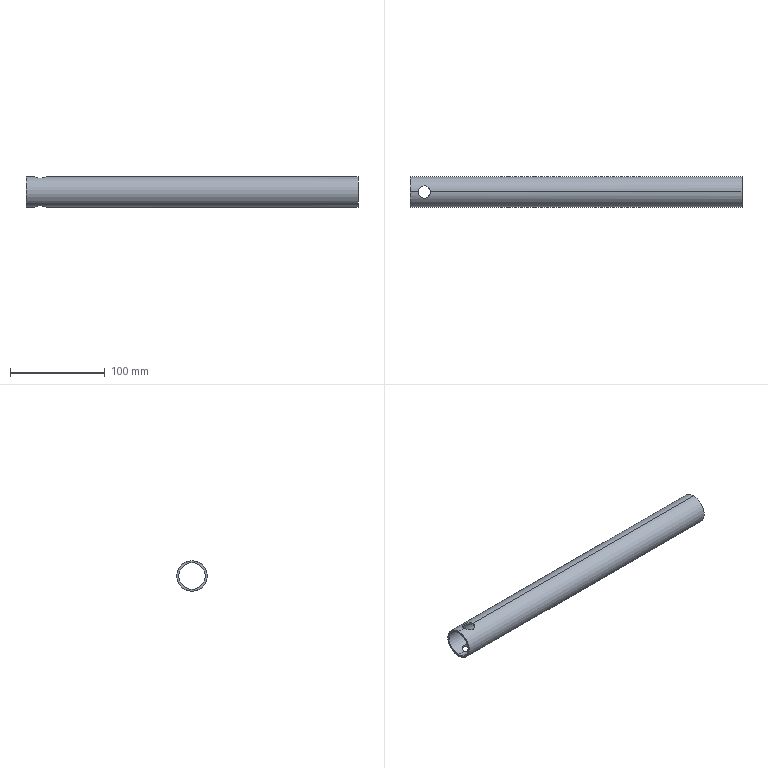Part | SolidWorks | features ICE 1, Sweep 1 | 1 solid | 10 faces | box 350 x 32 x 32 mm | volume 65429 mm3 | cylinder 8 | plane 2 | commonest cylinder face diameters 13 x4 28 x2 32 x2
STEP:
#1=CARTESIAN_POINT('',(-153.5,0.,-16.));
#2=VERTEX_POINT('',#1);
#3=CARTESIAN_POINT('',(-166.5,0.,-16.));
#4=VERTEX_POINT('',#3);
#5=CARTESIAN_POINT('',(-153.5,0.,-16.));
#6=CARTESIAN_POINT('',(-153.5,-0.4345,-16.));
#7=CARTESIAN_POINT('',(-153.543,-0.8609,-15.982));
#8=CARTESIAN_POINT('',(-153.669,-1.489,-15.932));
#9=CARTESIAN_POINT('',(-153.722,-1.696,-15.911));
#10=CARTESIAN_POINT('',(-153.847,-2.107,-15.862));
#11=CARTESIAN_POINT('',(-153.921,-2.31,-15.834));
#12=CARTESIAN_POINT('',(-154.167,-2.899,-15.74));
#13=CARTESIAN_POINT('',(-154.367,-3.271,-15.666));
#14=CARTESIAN_POINT('',(-154.721,-3.798,-15.544));
#15=CARTESIAN_POINT('',(-154.849,-3.97,-15.501));
#16=CARTESIAN_POINT('',(-155.117,-4.296,-15.413));
#17=CARTESIAN_POINT('',(-155.259,-4.451,-15.369));
#18=CARTESIAN_POINT('',(-155.703,-4.895,-15.236));
#19=CARTESIAN_POINT('',(-156.029,-5.164,-15.146));
#20=CARTESIAN_POINT('',(-156.735,-5.637,-14.976));
#21=CARTESIAN_POINT('',(-157.106,-5.836,-14.899));
#22=CARTESIAN_POINT('',(-157.691,-6.08,-14.8));
#23=CARTESIAN_POINT('',(-157.891,-6.152,-14.77));
#24=CARTESIAN_POINT('',(-158.3,-6.278,-14.717));
#25=CARTESIAN_POINT('',(-158.511,-6.331,-14.694));
#26=CARTESIAN_POINT('',(-159.142,-6.457,-14.639));
#27=CARTESIAN_POINT('',(-159.567,-6.5,-14.62));
#28=CARTESIAN_POINT('',(-160.425,-6.5,-14.62));
#29=CARTESIAN_POINT('',(-160.861,-6.457,-14.64));
#30=CARTESIAN_POINT('',(-161.699,-6.289,-14.713));
#31=CARTESIAN_POINT('',(-162.108,-6.164,-14.766));
#32=CARTESIAN_POINT('',(-162.899,-5.833,-14.9));
#33=CARTESIAN_POINT('',(-163.271,-5.633,-14.978));
#34=CARTESIAN_POINT('',(-163.97,-5.164,-15.146));
#35=CARTESIAN_POINT('',(-164.301,-4.892,-15.237));
#36=CARTESIAN_POINT('',(-164.895,-4.297,-15.415));
#37=CARTESIAN_POINT('',(-165.161,-3.973,-15.503));
#38=CARTESIAN_POINT('',(-165.515,-3.447,-15.625));
#39=CARTESIAN_POINT('',(-165.626,-3.263,-15.665));
#40=CARTESIAN_POINT('',(-165.827,-2.888,-15.738));
#41=CARTESIAN_POINT('',(-165.918,-2.697,-15.772));
#42=CARTESIAN_POINT('',(-166.162,-2.111,-15.865));
#43=CARTESIAN_POINT('',(-166.287,-1.704,-15.915));
#44=CARTESIAN_POINT('',(-166.458,-0.8569,-15.983));
#45=CARTESIAN_POINT('',(-166.5,-0.428,-16.));
#46=CARTESIAN_POINT('',(-166.5,0.,-16.));
#47=B_SPLINE_CURVE_WITH_KNOTS('',3,(#5,#6,#7,#8,#9,#10,#11,#12,#13,#14,#15,#16,#17,#18,#19,#20,#21,#22,#23,#24,#25,#26,#27,#28,#29,#30,#31,#32,#33,#34,#35,#36,#37,#38,#39,#40,#41,#42,#43,#44,#45,#46),.UNSPECIFIED.,.F.,.F.,(4,2,2,2,2,2,2,2,2,2,2,2,2,2,2,2,2,2,2,2,4),(0.,0.001284,0.001926,0.002568,0.003852,0.004495,0.005137,0.006421,0.007705,0.008347,0.008989,0.01027,0.01156,0.01284,0.01413,0.01541,0.01669,0.01734,0.01798,0.01926,0.02055),.UNSPECIFIED.);
#48=EDGE_CURVE('',#2,#4,#47,.T.);
#49=ORIENTED_EDGE('',*,*,#48,.T.);
#50=CARTESIAN_POINT('',(-166.5,0.,-14.));
#51=VERTEX_POINT('',#50);
#52=CARTESIAN_POINT('',(-166.5,0.,-16.));
#53=DIRECTION('',(0.,0.,1.));
#54=VECTOR('',#53,1000.);
#55=LINE('',#52,#54);
#56=EDGE_CURVE('',#4,#51,#55,.T.);
#57=ORIENTED_EDGE('',*,*,#56,.T.);
#58=CARTESIAN_POINT('',(-153.5,0.,-14.));
#59=VERTEX_POINT('',#58);
#60=CARTESIAN_POINT('',(-153.5,0.,-14.));
#61=CARTESIAN_POINT('',(-153.5,-0.4294,-14.));
#62=CARTESIAN_POINT('',(-153.544,-0.8664,-13.98));
#63=CARTESIAN_POINT('',(-153.714,-1.708,-13.902));
#64=CARTESIAN_POINT('',(-153.839,-2.116,-13.845));
#65=CARTESIAN_POINT('',(-154.087,-2.708,-13.737));
#66=CARTESIAN_POINT('',(-154.18,-2.902,-13.697));
#67=CARTESIAN_POINT('',(-154.381,-3.274,-13.613));
#68=CARTESIAN_POINT('',(-154.49,-3.454,-13.568));
#69=CARTESIAN_POINT('',(-154.724,-3.803,-13.475));
#70=CARTESIAN_POINT('',(-154.85,-3.971,-13.426));
#71=CARTESIAN_POINT('',(-155.118,-4.296,-13.326));
#72=CARTESIAN_POINT('',(-155.261,-4.453,-13.274));
#73=CARTESIAN_POINT('',(-155.706,-4.898,-13.119));
#74=CARTESIAN_POINT('',(-156.029,-5.163,-13.016));
#75=CARTESIAN_POINT('',(-156.726,-5.631,-12.82));
#76=CARTESIAN_POINT('',(-157.104,-5.834,-12.728));
#77=CARTESIAN_POINT('',(-157.883,-6.16,-12.573));
#78=CARTESIAN_POINT('',(-158.288,-6.285,-12.51));
#79=CARTESIAN_POINT('',(-158.921,-6.413,-12.445));
#80=CARTESIAN_POINT('',(-159.137,-6.446,-12.428));
#81=CARTESIAN_POINT('',(-159.566,-6.489,-12.405));
#82=CARTESIAN_POINT('',(-159.996,-6.511,-12.394));
#83=CARTESIAN_POINT('',(-160.424,-6.49,-12.405));
#84=CARTESIAN_POINT('',(-160.853,-6.447,-12.427));
#85=CARTESIAN_POINT('',(-161.068,-6.415,-12.444));
#86=CARTESIAN_POINT('',(-161.704,-6.288,-12.509));
#87=CARTESIAN_POINT('',(-162.111,-6.162,-12.572));
#88=CARTESIAN_POINT('',(-162.895,-5.835,-12.727));
#89=CARTESIAN_POINT('',(-163.273,-5.632,-12.82));
#90=CARTESIAN_POINT('',(-163.97,-5.164,-13.015));
#91=CARTESIAN_POINT('',(-164.294,-4.898,-13.119));
#92=CARTESIAN_POINT('',(-164.892,-4.301,-13.327));
#93=CARTESIAN_POINT('',(-165.158,-3.978,-13.428));
#94=CARTESIAN_POINT('',(-165.509,-3.456,-13.568));
#95=CARTESIAN_POINT('',(-165.618,-3.276,-13.613));
#96=CARTESIAN_POINT('',(-165.82,-2.902,-13.697));
#97=CARTESIAN_POINT('',(-165.913,-2.708,-13.737));
#98=CARTESIAN_POINT('',(-166.16,-2.118,-13.845));
#99=CARTESIAN_POINT('',(-166.285,-1.712,-13.901));
#100=CARTESIAN_POINT('',(-166.455,-0.8727,-13.979));
#101=CARTESIAN_POINT('',(-166.5,-0.4357,-14.));
#102=CARTESIAN_POINT('',(-166.5,0.,-14.));
#103=B_SPLINE_CURVE_WITH_KNOTS('',3,(#60,#61,#62,#63,#64,#65,#66,#67,#68,#69,#70,#71,#72,#73,#74,#75,#76,#77,#78,#79,#80,#81,#82,#83,#84,#85,#86,#87,#88,#89,#90,#91,#92,#93,#94,#95,#96,#97,#98,#99,#100,#101,#102),.UNSPECIFIED.,.F.,.F.,(4,2,2,2,2,2,2,2,2,2,2,1,2,2,2,2,2,2,2,2,2,4),(0.02062,0.02191,0.0232,0.02384,0.02448,0.02513,0.02577,0.02706,0.02835,0.02963,0.03028,0.03092,0.03156,0.03221,0.03349,0.03478,0.03607,0.03736,0.038,0.03864,0.03993,0.04122),.UNSPECIFIED.);
#104=EDGE_CURVE('',#59,#51,#103,.T.);
#105=ORIENTED_EDGE('',*,*,#104,.F.);
#106=CARTESIAN_POINT('',(-153.5,0.,-16.));
#107=DIRECTION('',(0.,0.,1.));
#108=VECTOR('',#107,1000.);
#109=LINE('',#106,#108);
#110=EDGE_CURVE('',#2,#59,#109,.T.);
#111=ORIENTED_EDGE('',*,*,#110,.F.);
#112=EDGE_LOOP('',(#49,#57,#105,#111));
#113=FACE_OUTER_BOUND('',#112,.T.);
#114=CARTESIAN_POINT('',(-160.,0.,-16.));
#115=DIRECTION('',(0.,0.,1.));
#116=DIRECTION('',(1.,0.,0.));
#117=AXIS2_PLACEMENT_3D('',#114,#115,#116);
#118=CYLINDRICAL_SURFACE('',#117,6.5);
#119=ADVANCED_FACE('',(#113),#118,.F.);
#120=CARTESIAN_POINT('',(-166.5,0.,14.));
#121=VERTEX_POINT('',#120);
#122=CARTESIAN_POINT('',(-153.5,0.,14.));
#123=VERTEX_POINT('',#122);
#124=CARTESIAN_POINT('',(-166.5,0.,14.));
#125=CARTESIAN_POINT('',(-166.5,-0.4294,14.));
#126=CARTESIAN_POINT('',(-166.456,-0.8664,13.98));
#127=CARTESIAN_POINT('',(-166.286,-1.708,13.902));
#128=CARTESIAN_POINT('',(-166.161,-2.116,13.845));
#129=CARTESIAN_POINT('',(-165.913,-2.708,13.737));
#130=CARTESIAN_POINT('',(-165.82,-2.902,13.697));
#131=CARTESIAN_POINT('',(-165.619,-3.274,13.613));
#132=CARTESIAN_POINT('',(-165.51,-3.454,13.568));
#133=CARTESIAN_POINT('',(-165.276,-3.803,13.475));
#134=CARTESIAN_POINT('',(-165.15,-3.971,13.426));
#135=CARTESIAN_POINT('',(-164.882,-4.296,13.326));
#136=CARTESIAN_POINT('',(-164.739,-4.453,13.274));
#137=CARTESIAN_POINT('',(-164.294,-4.898,13.119));
#138=CARTESIAN_POINT('',(-163.971,-5.163,13.016));
#139=CARTESIAN_POINT('',(-163.274,-5.631,12.82));
#140=CARTESIAN_POINT('',(-162.896,-5.834,12.728));
#141=CARTESIAN_POINT('',(-162.117,-6.16,12.573));
#142=CARTESIAN_POINT('',(-161.712,-6.285,12.51));
#143=CARTESIAN_POINT('',(-161.079,-6.413,12.445));
#144=CARTESIAN_POINT('',(-160.863,-6.446,12.428));
#145=CARTESIAN_POINT('',(-160.434,-6.489,12.405));
#146=CARTESIAN_POINT('',(-160.004,-6.511,12.394));
#147=CARTESIAN_POINT('',(-159.576,-6.49,12.405));
#148=CARTESIAN_POINT('',(-159.147,-6.447,12.427));
#149=CARTESIAN_POINT('',(-158.932,-6.415,12.444));
#150=CARTESIAN_POINT('',(-158.296,-6.288,12.509));
#151=CARTESIAN_POINT('',(-157.889,-6.162,12.572));
#152=CARTESIAN_POINT('',(-157.105,-5.835,12.727));
#153=CARTESIAN_POINT('',(-156.727,-5.632,12.82));
#154=CARTESIAN_POINT('',(-156.03,-5.164,13.015));
#155=CARTESIAN_POINT('',(-155.706,-4.898,13.119));
#156=CARTESIAN_POINT('',(-155.108,-4.301,13.327));
#157=CARTESIAN_POINT('',(-154.842,-3.978,13.428));
#158=CARTESIAN_POINT('',(-154.491,-3.456,13.568));
#159=CARTESIAN_POINT('',(-154.382,-3.276,13.613));
#160=CARTESIAN_POINT('',(-154.18,-2.902,13.697));
#161=CARTESIAN_POINT('',(-154.087,-2.708,13.737));
#162=CARTESIAN_POINT('',(-153.84,-2.118,13.845));
#163=CARTESIAN_POINT('',(-153.715,-1.712,13.901));
#164=CARTESIAN_POINT('',(-153.545,-0.8727,13.979));
#165=CARTESIAN_POINT('',(-153.5,-0.4357,14.));
#166=CARTESIAN_POINT('',(-153.5,0.,14.));
#167=B_SPLINE_CURVE_WITH_KNOTS('',3,(#124,#125,#126,#127,#128,#129,#130,#131,#132,#133,#134,#135,#136,#137,#138,#139,#140,#141,#142,#143,#144,#145,#146,#147,#148,#149,#150,#151,#152,#153,#154,#155,#156,#157,#158,#159,#160,#161,#162,#163,#164,#165,#166),.UNSPECIFIED.,.F.,.F.,(4,2,2,2,2,2,2,2,2,2,2,1,2,2,2,2,2,2,2,2,2,4),(0.02062,0.02191,0.0232,0.02384,0.02448,0.02513,0.02577,0.02706,0.02835,0.02963,0.03028,0.03092,0.03156,0.03221,0.03349,0.03478,0.03607,0.03736,0.038,0.03864,0.03993,0.04122),.UNSPECIFIED.);
#168=EDGE_CURVE('',#121,#123,#167,.T.);
#169=ORIENTED_EDGE('',*,*,#168,.F.);
#170=CARTESIAN_POINT('',(-166.5,0.,16.));
#171=VERTEX_POINT('',#170);
#172=CARTESIAN_POINT('',(-166.5,0.,-16.));
#173=DIRECTION('',(0.,0.,1.));
#174=VECTOR('',#173,1000.);
#175=LINE('',#172,#174);
#176=EDGE_CURVE('',#121,#171,#175,.T.);
#177=ORIENTED_EDGE('',*,*,#176,.T.);
#178=CARTESIAN_POINT('',(-153.5,0.,16.));
#179=VERTEX_POINT('',#178);
#180=CARTESIAN_POINT('',(-166.5,0.,16.));
#181=CARTESIAN_POINT('',(-166.5,-0.2139,16.));
#182=CARTESIAN_POINT('',(-166.489,-0.428,15.996));
#183=CARTESIAN_POINT('',(-166.447,-0.8567,15.978));
#184=CARTESIAN_POINT('',(-166.415,-1.072,15.965));
#185=CARTESIAN_POINT('',(-166.287,-1.704,15.915));
#186=CARTESIAN_POINT('',(-166.163,-2.111,15.865));
#187=CARTESIAN_POINT('',(-165.916,-2.701,15.772));
#188=CARTESIAN_POINT('',(-165.824,-2.895,15.737));
#189=CARTESIAN_POINT('',(-165.622,-3.269,15.664));
#190=CARTESIAN_POINT('',(-165.513,-3.45,15.625));
#191=CARTESIAN_POINT('',(-165.161,-3.974,15.503));
#192=CARTESIAN_POINT('',(-164.892,-4.301,15.414));
#193=CARTESIAN_POINT('',(-164.293,-4.899,15.235));
#194=CARTESIAN_POINT('',(-163.969,-5.165,15.145));
#195=CARTESIAN_POINT('',(-163.445,-5.516,15.02));
#196=CARTESIAN_POINT('',(-163.265,-5.625,14.979));
#197=CARTESIAN_POINT('',(-162.89,-5.826,14.902));
#198=CARTESIAN_POINT('',(-162.697,-5.918,14.866));
#199=CARTESIAN_POINT('',(-162.109,-6.163,14.766));
#200=CARTESIAN_POINT('',(-161.703,-6.287,14.713));
#201=CARTESIAN_POINT('',(-160.865,-6.456,14.64));
#202=CARTESIAN_POINT('',(-160.43,-6.5,14.62));
#203=CARTESIAN_POINT('',(-159.573,-6.5,14.62));
#204=CARTESIAN_POINT('',(-159.147,-6.458,14.639));
#205=CARTESIAN_POINT('',(-158.3,-6.288,14.713));
#206=CARTESIAN_POINT('',(-157.89,-6.163,14.767));
#207=CARTESIAN_POINT('',(-157.108,-5.836,14.899));
#208=CARTESIAN_POINT('',(-156.729,-5.633,14.978));
#209=CARTESIAN_POINT('',(-156.028,-5.163,15.146));
#210=CARTESIAN_POINT('',(-155.704,-4.897,15.236));
#211=CARTESIAN_POINT('',(-155.257,-4.449,15.37));
#212=CARTESIAN_POINT('',(-155.114,-4.292,15.415));
#213=CARTESIAN_POINT('',(-154.845,-3.965,15.502));
#214=CARTESIAN_POINT('',(-154.72,-3.797,15.544));
#215=CARTESIAN_POINT('',(-154.369,-3.273,15.666));
#216=CARTESIAN_POINT('',(-154.168,-2.902,15.74));
#217=CARTESIAN_POINT('',(-153.837,-2.109,15.865));
#218=CARTESIAN_POINT('',(-153.712,-1.701,15.915));
#219=CARTESIAN_POINT('',(-153.586,-1.075,15.965));
#220=CARTESIAN_POINT('',(-153.554,-0.8632,15.978));
#221=CARTESIAN_POINT('',(-153.511,-0.4349,15.996));
#222=CARTESIAN_POINT('',(-153.5,-0.2171,16.));
#223=CARTESIAN_POINT('',(-153.5,0.,16.));
#224=B_SPLINE_CURVE_WITH_KNOTS('',3,(#180,#181,#182,#183,#184,#185,#186,#187,#188,#189,#190,#191,#192,#193,#194,#195,#196,#197,#198,#199,#200,#201,#202,#203,#204,#205,#206,#207,#208,#209,#210,#211,#212,#213,#214,#215,#216,#217,#218,#219,#220,#221,#222,#223),.UNSPECIFIED.,.F.,.F.,(4,2,2,2,2,2,2,2,2,2,2,2,2,2,2,2,2,2,2,2,2,4),(0.02055,0.02119,0.02183,0.02311,0.02375,0.0244,0.02568,0.02696,0.0276,0.02825,0.02953,0.03081,0.0321,0.03338,0.03466,0.03595,0.03659,0.03723,0.03851,0.0398,0.04044,0.04108),.UNSPECIFIED.);
#225=EDGE_CURVE('',#171,#179,#224,.T.);
#226=ORIENTED_EDGE('',*,*,#225,.T.);
#227=CARTESIAN_POINT('',(-153.5,0.,-16.));
#228=DIRECTION('',(0.,0.,1.));
#229=VECTOR('',#228,1000.);
#230=LINE('',#227,#229);
#231=EDGE_CURVE('',#123,#179,#230,.T.);
#232=ORIENTED_EDGE('',*,*,#231,.F.);
#233=EDGE_LOOP('',(#169,#177,#226,#232));
#234=FACE_OUTER_BOUND('',#233,.T.);
#235=CARTESIAN_POINT('',(-160.,0.,-16.));
#236=DIRECTION('',(0.,0.,1.));
#237=DIRECTION('',(1.,0.,0.));
#238=AXIS2_PLACEMENT_3D('',#235,#236,#237);
#239=CYLINDRICAL_SURFACE('',#238,6.5);
#240=ADVANCED_FACE('',(#234),#239,.F.);
#241=CARTESIAN_POINT('',(-175.,0.,14.));
#242=VERTEX_POINT('',#241);
#243=CARTESIAN_POINT('',(-175.,0.,-14.));
#244=VERTEX_POINT('',#243);
#245=CARTESIAN_POINT('',(-175.,0.,0.));
#246=DIRECTION('',(1.,0.,0.));
#247=DIRECTION('',(0.,0.,-1.));
#248=AXIS2_PLACEMENT_3D('',#245,#246,#247);
#249=CIRCLE('',#248,14.);
#250=EDGE_CURVE('',#242,#244,#249,.T.);
#251=ORIENTED_EDGE('',*,*,#250,.F.);
#252=CARTESIAN_POINT('',(-175.,0.,14.));
#253=DIRECTION('',(1.,0.,0.));
#254=VECTOR('',#253,1000.);
#255=LINE('',#252,#254);
#256=EDGE_CURVE('',#242,#121,#255,.T.);
#257=ORIENTED_EDGE('',*,*,#256,.T.);
#258=ORIENTED_EDGE('',*,*,#168,.T.);
#259=CARTESIAN_POINT('',(175.,0.,14.));
#260=VERTEX_POINT('',#259);
#261=CARTESIAN_POINT('',(-175.,0.,14.));
#262=DIRECTION('',(1.,0.,0.));
#263=VECTOR('',#262,1000.);
#264=LINE('',#261,#263);
#265=EDGE_CURVE('',#123,#260,#264,.T.);
#266=ORIENTED_EDGE('',*,*,#265,.T.);
#267=CARTESIAN_POINT('',(175.,0.,-14.));
#268=VERTEX_POINT('',#267);
#269=CARTESIAN_POINT('',(175.,0.,0.));
#270=DIRECTION('',(1.,0.,0.));
#271=DIRECTION('',(0.,0.,-1.));
#272=AXIS2_PLACEMENT_3D('',#269,#270,#271);
#273=CIRCLE('',#272,14.);
#274=EDGE_CURVE('',#260,#268,#273,.T.);
#275=ORIENTED_EDGE('',*,*,#274,.T.);
#276=CARTESIAN_POINT('',(-175.,0.,-14.));
#277=DIRECTION('',(1.,0.,0.));
#278=VECTOR('',#277,1000.);
#279=LINE('',#276,#278);
#280=EDGE_CURVE('',#59,#268,#279,.T.);
#281=ORIENTED_EDGE('',*,*,#280,.F.);
#282=ORIENTED_EDGE('',*,*,#104,.T.);
#283=CARTESIAN_POINT('',(-175.,0.,-14.));
#284=DIRECTION('',(1.,0.,0.));
#285=VECTOR('',#284,1000.);
#286=LINE('',#283,#285);
#287=EDGE_CURVE('',#244,#51,#286,.T.);
#288=ORIENTED_EDGE('',*,*,#287,.F.);
#289=EDGE_LOOP('',(#251,#257,#258,#266,#275,#281,#282,#288));
#290=FACE_OUTER_BOUND('',#289,.T.);
#291=CARTESIAN_POINT('',(-175.,0.,0.));
#292=DIRECTION('',(1.,0.,0.));
#293=DIRECTION('',(0.,0.,-1.));
#294=AXIS2_PLACEMENT_3D('',#291,#292,#293);
#295=CYLINDRICAL_SURFACE('',#294,14.);
#296=ADVANCED_FACE('',(#290),#295,.F.);
#297=CARTESIAN_POINT('',(-175.,0.,-16.));
#298=VERTEX_POINT('',#297);
#299=CARTESIAN_POINT('',(-175.,0.,16.));
#300=VERTEX_POINT('',#299);
#301=CARTESIAN_POINT('',(-175.,0.,0.));
#302=DIRECTION('',(1.,0.,0.));
#303=DIRECTION('',(0.,0.,-1.));
#304=AXIS2_PLACEMENT_3D('',#301,#302,#303);
#305=CIRCLE('',#304,16.);
#306=EDGE_CURVE('',#298,#300,#305,.T.);
#307=ORIENTED_EDGE('',*,*,#306,.T.);
#308=CARTESIAN_POINT('',(-175.,0.,16.));
#309=DIRECTION('',(1.,0.,0.));
#310=VECTOR('',#309,1000.);
#311=LINE('',#308,#310);
#312=EDGE_CURVE('',#300,#171,#311,.T.);
#313=ORIENTED_EDGE('',*,*,#312,.T.);
#314=CARTESIAN_POINT('',(-153.5,0.,16.));
#315=CARTESIAN_POINT('',(-153.5,0.4345,16.));
#316=CARTESIAN_POINT('',(-153.543,0.8609,15.982));
#317=CARTESIAN_POINT('',(-153.669,1.489,15.932));
#318=CARTESIAN_POINT('',(-153.722,1.696,15.911));
#319=CARTESIAN_POINT('',(-153.847,2.107,15.862));
#320=CARTESIAN_POINT('',(-153.921,2.31,15.834));
#321=CARTESIAN_POINT('',(-154.167,2.899,15.74));
#322=CARTESIAN_POINT('',(-154.367,3.271,15.666));
#323=CARTESIAN_POINT('',(-154.721,3.798,15.544));
#324=CARTESIAN_POINT('',(-154.849,3.97,15.501));
#325=CARTESIAN_POINT('',(-155.117,4.296,15.413));
#326=CARTESIAN_POINT('',(-155.259,4.451,15.369));
#327=CARTESIAN_POINT('',(-155.703,4.895,15.236));
#328=CARTESIAN_POINT('',(-156.029,5.164,15.146));
#329=CARTESIAN_POINT('',(-156.735,5.637,14.976));
#330=CARTESIAN_POINT('',(-157.106,5.836,14.899));
#331=CARTESIAN_POINT('',(-157.691,6.08,14.8));
#332=CARTESIAN_POINT('',(-157.891,6.152,14.77));
#333=CARTESIAN_POINT('',(-158.3,6.278,14.717));
#334=CARTESIAN_POINT('',(-158.511,6.331,14.694));
#335=CARTESIAN_POINT('',(-159.142,6.457,14.639));
#336=CARTESIAN_POINT('',(-159.567,6.5,14.62));
#337=CARTESIAN_POINT('',(-160.425,6.5,14.62));
#338=CARTESIAN_POINT('',(-160.861,6.457,14.64));
#339=CARTESIAN_POINT('',(-161.699,6.289,14.713));
#340=CARTESIAN_POINT('',(-162.108,6.164,14.766));
#341=CARTESIAN_POINT('',(-162.899,5.833,14.9));
#342=CARTESIAN_POINT('',(-163.271,5.633,14.978));
#343=CARTESIAN_POINT('',(-163.97,5.164,15.146));
#344=CARTESIAN_POINT('',(-164.301,4.892,15.237));
#345=CARTESIAN_POINT('',(-164.895,4.297,15.415));
#346=CARTESIAN_POINT('',(-165.161,3.973,15.503));
#347=CARTESIAN_POINT('',(-165.515,3.447,15.625));
#348=CARTESIAN_POINT('',(-165.626,3.263,15.665));
#349=CARTESIAN_POINT('',(-165.827,2.888,15.738));
#350=CARTESIAN_POINT('',(-165.918,2.697,15.772));
#351=CARTESIAN_POINT('',(-166.162,2.111,15.865));
#352=CARTESIAN_POINT('',(-166.287,1.704,15.915));
#353=CARTESIAN_POINT('',(-166.458,0.8569,15.983));
#354=CARTESIAN_POINT('',(-166.5,0.428,16.));
#355=CARTESIAN_POINT('',(-166.5,0.,16.));
#356=B_SPLINE_CURVE_WITH_KNOTS('',3,(#314,#315,#316,#317,#318,#319,#320,#321,#322,#323,#324,#325,#326,#327,#328,#329,#330,#331,#332,#333,#334,#335,#336,#337,#338,#339,#340,#341,#342,#343,#344,#345,#346,#347,#348,#349,#350,#351,#352,#353,#354,#355),.UNSPECIFIED.,.F.,.F.,(4,2,2,2,2,2,2,2,2,2,2,2,2,2,2,2,2,2,2,2,4),(0.,0.001284,0.001926,0.002568,0.003852,0.004495,0.005137,0.006421,0.007705,0.008347,0.008989,0.01027,0.01156,0.01284,0.01413,0.01541,0.01669,0.01734,0.01798,0.01926,0.02055),.UNSPECIFIED.);
#357=EDGE_CURVE('',#179,#171,#356,.T.);
#358=ORIENTED_EDGE('',*,*,#357,.F.);
#359=CARTESIAN_POINT('',(175.,0.,16.));
#360=VERTEX_POINT('',#359);
#361=CARTESIAN_POINT('',(-175.,0.,16.));
#362=DIRECTION('',(1.,0.,0.));
#363=VECTOR('',#362,1000.);
#364=LINE('',#361,#363);
#365=EDGE_CURVE('',#179,#360,#364,.T.);
#366=ORIENTED_EDGE('',*,*,#365,.T.);
#367=CARTESIAN_POINT('',(175.,0.,-16.));
#368=VERTEX_POINT('',#367);
#369=CARTESIAN_POINT('',(175.,0.,0.));
#370=DIRECTION('',(1.,0.,0.));
#371=DIRECTION('',(0.,0.,-1.));
#372=AXIS2_PLACEMENT_3D('',#369,#370,#371);
#373=CIRCLE('',#372,16.);
#374=EDGE_CURVE('',#368,#360,#373,.T.);
#375=ORIENTED_EDGE('',*,*,#374,.F.);
#376=CARTESIAN_POINT('',(-175.,0.,-16.));
#377=DIRECTION('',(1.,0.,0.));
#378=VECTOR('',#377,1000.);
#379=LINE('',#376,#378);
#380=EDGE_CURVE('',#2,#368,#379,.T.);
#381=ORIENTED_EDGE('',*,*,#380,.F.);
#382=CARTESIAN_POINT('',(-166.5,0.,-16.));
#383=CARTESIAN_POINT('',(-166.5,0.2139,-16.));
#384=CARTESIAN_POINT('',(-166.489,0.428,-15.996));
#385=CARTESIAN_POINT('',(-166.447,0.8567,-15.978));
#386=CARTESIAN_POINT('',(-166.415,1.072,-15.965));
#387=CARTESIAN_POINT('',(-166.287,1.704,-15.915));
#388=CARTESIAN_POINT('',(-166.163,2.111,-15.865));
#389=CARTESIAN_POINT('',(-165.916,2.701,-15.772));
#390=CARTESIAN_POINT('',(-165.824,2.895,-15.737));
#391=CARTESIAN_POINT('',(-165.622,3.269,-15.664));
#392=CARTESIAN_POINT('',(-165.513,3.45,-15.625));
#393=CARTESIAN_POINT('',(-165.161,3.974,-15.503));
#394=CARTESIAN_POINT('',(-164.892,4.301,-15.414));
#395=CARTESIAN_POINT('',(-164.293,4.899,-15.235));
#396=CARTESIAN_POINT('',(-163.969,5.165,-15.145));
#397=CARTESIAN_POINT('',(-163.445,5.516,-15.02));
#398=CARTESIAN_POINT('',(-163.265,5.625,-14.979));
#399=CARTESIAN_POINT('',(-162.89,5.826,-14.902));
#400=CARTESIAN_POINT('',(-162.697,5.918,-14.866));
#401=CARTESIAN_POINT('',(-162.109,6.163,-14.766));
#402=CARTESIAN_POINT('',(-161.703,6.287,-14.713));
#403=CARTESIAN_POINT('',(-160.865,6.456,-14.64));
#404=CARTESIAN_POINT('',(-160.43,6.5,-14.62));
#405=CARTESIAN_POINT('',(-159.573,6.5,-14.62));
#406=CARTESIAN_POINT('',(-159.147,6.458,-14.639));
#407=CARTESIAN_POINT('',(-158.3,6.288,-14.713));
#408=CARTESIAN_POINT('',(-157.89,6.163,-14.767));
#409=CARTESIAN_POINT('',(-157.108,5.836,-14.899));
#410=CARTESIAN_POINT('',(-156.729,5.633,-14.978));
#411=CARTESIAN_POINT('',(-156.028,5.163,-15.146));
#412=CARTESIAN_POINT('',(-155.704,4.897,-15.236));
#413=CARTESIAN_POINT('',(-155.257,4.449,-15.37));
#414=CARTESIAN_POINT('',(-155.114,4.292,-15.415));
#415=CARTESIAN_POINT('',(-154.845,3.965,-15.502));
#416=CARTESIAN_POINT('',(-154.72,3.797,-15.544));
#417=CARTESIAN_POINT('',(-154.369,3.273,-15.666));
#418=CARTESIAN_POINT('',(-154.168,2.902,-15.74));
#419=CARTESIAN_POINT('',(-153.837,2.109,-15.865));
#420=CARTESIAN_POINT('',(-153.712,1.701,-15.915));
#421=CARTESIAN_POINT('',(-153.586,1.075,-15.965));
#422=CARTESIAN_POINT('',(-153.554,0.8632,-15.978));
#423=CARTESIAN_POINT('',(-153.511,0.4349,-15.996));
#424=CARTESIAN_POINT('',(-153.5,0.2171,-16.));
#425=CARTESIAN_POINT('',(-153.5,0.,-16.));
#426=B_SPLINE_CURVE_WITH_KNOTS('',3,(#382,#383,#384,#385,#386,#387,#388,#389,#390,#391,#392,#393,#394,#395,#396,#397,#398,#399,#400,#401,#402,#403,#404,#405,#406,#407,#408,#409,#410,#411,#412,#413,#414,#415,#416,#417,#418,#419,#420,#421,#422,#423,#424,#425),.UNSPECIFIED.,.F.,.F.,(4,2,2,2,2,2,2,2,2,2,2,2,2,2,2,2,2,2,2,2,2,4),(0.02055,0.02119,0.02183,0.02311,0.02375,0.0244,0.02568,0.02696,0.0276,0.02825,0.02953,0.03081,0.0321,0.03338,0.03466,0.03595,0.03659,0.03723,0.03851,0.0398,0.04044,0.04108),.UNSPECIFIED.);
#427=EDGE_CURVE('',#4,#2,#426,.T.);
#428=ORIENTED_EDGE('',*,*,#427,.F.);
#429=CARTESIAN_POINT('',(-175.,0.,-16.));
#430=DIRECTION('',(1.,0.,0.));
#431=VECTOR('',#430,1000.);
#432=LINE('',#429,#431);
#433=EDGE_CURVE('',#298,#4,#432,.T.);
#434=ORIENTED_EDGE('',*,*,#433,.F.);
#435=EDGE_LOOP('',(#307,#313,#358,#366,#375,#381,#428,#434));
#436=FACE_OUTER_BOUND('',#435,.T.);
#437=CARTESIAN_POINT('',(-175.,0.,0.));
#438=DIRECTION('',(1.,0.,0.));
#439=DIRECTION('',(0.,0.,-1.));
#440=AXIS2_PLACEMENT_3D('',#437,#438,#439);
#441=CYLINDRICAL_SURFACE('',#440,16.);
#442=ADVANCED_FACE('',(#436),#441,.T.);
#443=ORIENTED_EDGE('',*,*,#312,.F.);
#444=CARTESIAN_POINT('',(-175.,0.,0.));
#445=DIRECTION('',(1.,0.,0.));
#446=DIRECTION('',(0.,0.,-1.));
#447=AXIS2_PLACEMENT_3D('',#444,#445,#446);
#448=CIRCLE('',#447,16.);
#449=EDGE_CURVE('',#300,#298,#448,.T.);
#450=ORIENTED_EDGE('',*,*,#449,.T.);
#451=ORIENTED_EDGE('',*,*,#433,.T.);
#452=ORIENTED_EDGE('',*,*,#48,.F.);
#453=ORIENTED_EDGE('',*,*,#380,.T.);
#454=CARTESIAN_POINT('',(175.,0.,0.));
#455=DIRECTION('',(1.,0.,0.));
#456=DIRECTION('',(0.,0.,-1.));
#457=AXIS2_PLACEMENT_3D('',#454,#455,#456);
#458=CIRCLE('',#457,16.);
#459=EDGE_CURVE('',#360,#368,#458,.T.);
#460=ORIENTED_EDGE('',*,*,#459,.F.);
#461=ORIENTED_EDGE('',*,*,#365,.F.);
#462=ORIENTED_EDGE('',*,*,#225,.F.);
#463=EDGE_LOOP('',(#443,#450,#451,#452,#453,#460,#461,#462));
#464=FACE_OUTER_BOUND('',#463,.T.);
#465=CARTESIAN_POINT('',(-175.,0.,0.));
#466=DIRECTION('',(1.,0.,0.));
#467=DIRECTION('',(0.,0.,-1.));
#468=AXIS2_PLACEMENT_3D('',#465,#466,#467);
#469=CYLINDRICAL_SURFACE('',#468,16.);
#470=ADVANCED_FACE('',(#464),#469,.T.);
#471=CARTESIAN_POINT('',(175.,0.,0.));
#472=DIRECTION('',(1.,0.,0.));
#473=DIRECTION('',(0.,0.,-1.));
#474=AXIS2_PLACEMENT_3D('',#471,#472,#473);
#475=CIRCLE('',#474,14.);
#476=EDGE_CURVE('',#268,#260,#475,.T.);
#477=ORIENTED_EDGE('',*,*,#476,.F.);
#478=ORIENTED_EDGE('',*,*,#274,.F.);
#479=EDGE_LOOP('',(#477,#478));
#480=FACE_BOUND('',#479,.T.);
#481=ORIENTED_EDGE('',*,*,#374,.T.);
#482=ORIENTED_EDGE('',*,*,#459,.T.);
#483=EDGE_LOOP('',(#481,#482));
#484=FACE_OUTER_BOUND('',#483,.T.);
#485=CARTESIAN_POINT('',(175.,0.,0.));
#486=DIRECTION('',(1.,0.,0.));
#487=DIRECTION('',(0.,0.,-1.));
#488=AXIS2_PLACEMENT_3D('',#485,#486,#487);
#489=PLANE('',#488);
#490=ADVANCED_FACE('',(#480,#484),#489,.T.);
#491=CARTESIAN_POINT('',(-175.,0.,0.));
#492=DIRECTION('',(1.,0.,0.));
#493=DIRECTION('',(0.,0.,-1.));
#494=AXIS2_PLACEMENT_3D('',#491,#492,#493);
#495=CIRCLE('',#494,14.);
#496=EDGE_CURVE('',#244,#242,#495,.T.);
#497=ORIENTED_EDGE('',*,*,#496,.T.);
#498=ORIENTED_EDGE('',*,*,#250,.T.);
#499=EDGE_LOOP('',(#497,#498));
#500=FACE_BOUND('',#499,.T.);
#501=ORIENTED_EDGE('',*,*,#306,.F.);
#502=ORIENTED_EDGE('',*,*,#449,.F.);
#503=EDGE_LOOP('',(#501,#502));
#504=FACE_OUTER_BOUND('',#503,.T.);
#505=CARTESIAN_POINT('',(-175.,0.,0.));
#506=DIRECTION('',(1.,0.,0.));
#507=DIRECTION('',(0.,0.,-1.));
#508=AXIS2_PLACEMENT_3D('',#505,#506,#507);
#509=PLANE('',#508);
#510=ADVANCED_FACE('',(#500,#504),#509,.F.);
#511=ORIENTED_EDGE('',*,*,#256,.F.);
#512=ORIENTED_EDGE('',*,*,#496,.F.);
#513=ORIENTED_EDGE('',*,*,#287,.T.);
#514=CARTESIAN_POINT('',(-166.5,0.,-14.));
#515=CARTESIAN_POINT('',(-166.5,0.4362,-14.));
#516=CARTESIAN_POINT('',(-166.457,0.864,-13.98));
#517=CARTESIAN_POINT('',(-166.287,1.704,-13.902));
#518=CARTESIAN_POINT('',(-166.159,2.12,-13.844));
#519=CARTESIAN_POINT('',(-165.83,2.905,-13.701));
#520=CARTESIAN_POINT('',(-165.63,3.276,-13.616));
#521=CARTESIAN_POINT('',(-165.276,3.803,-13.475));
#522=CARTESIAN_POINT('',(-165.148,3.974,-13.425));
#523=CARTESIAN_POINT('',(-164.881,4.298,-13.325));
#524=CARTESIAN_POINT('',(-164.74,4.453,-13.274));
#525=CARTESIAN_POINT('',(-164.444,4.748,-13.171));
#526=CARTESIAN_POINT('',(-164.289,4.888,-13.12));
#527=CARTESIAN_POINT('',(-163.965,5.155,-13.017));
#528=CARTESIAN_POINT('',(-163.795,5.281,-12.966));
#529=CARTESIAN_POINT('',(-163.268,5.634,-12.819));
#530=CARTESIAN_POINT('',(-162.899,5.833,-12.728));
#531=CARTESIAN_POINT('',(-162.314,6.078,-12.612));
#532=CARTESIAN_POINT('',(-162.114,6.15,-12.577));
#533=CARTESIAN_POINT('',(-161.704,6.276,-12.515));
#534=CARTESIAN_POINT('',(-161.494,6.33,-12.487));
#535=CARTESIAN_POINT('',(-160.862,6.457,-12.423));
#536=CARTESIAN_POINT('',(-160.436,6.5,-12.4));
#537=CARTESIAN_POINT('',(-159.79,6.5,-12.4));
#538=CARTESIAN_POINT('',(-159.571,6.489,-12.405));
#539=CARTESIAN_POINT('',(-159.14,6.446,-12.428));
#540=CARTESIAN_POINT('',(-158.927,6.414,-12.444));
#541=CARTESIAN_POINT('',(-158.507,6.33,-12.487));
#542=CARTESIAN_POINT('',(-158.3,6.277,-12.514));
#543=CARTESIAN_POINT('',(-157.891,6.152,-12.576));
#544=CARTESIAN_POINT('',(-157.688,6.079,-12.612));
#545=CARTESIAN_POINT('',(-157.097,5.831,-12.729));
#546=CARTESIAN_POINT('',(-156.726,5.631,-12.82));
#547=CARTESIAN_POINT('',(-156.028,5.162,-13.016));
#548=CARTESIAN_POINT('',(-155.699,4.891,-13.121));
#549=CARTESIAN_POINT('',(-155.107,4.3,-13.327));
#550=CARTESIAN_POINT('',(-154.841,3.977,-13.428));
#551=CARTESIAN_POINT('',(-154.487,3.45,-13.57));
#552=CARTESIAN_POINT('',(-154.376,3.266,-13.615));
#553=CARTESIAN_POINT('',(-154.176,2.894,-13.699));
#554=CARTESIAN_POINT('',(-154.085,2.703,-13.738));
#555=CARTESIAN_POINT('',(-153.84,2.118,-13.845));
#556=CARTESIAN_POINT('',(-153.713,1.708,-13.902));
#557=CARTESIAN_POINT('',(-153.542,0.8576,-13.98));
#558=CARTESIAN_POINT('',(-153.5,0.43,-14.));
#559=CARTESIAN_POINT('',(-153.5,0.,-14.));
#560=B_SPLINE_CURVE_WITH_KNOTS('',3,(#514,#515,#516,#517,#518,#519,#520,#521,#522,#523,#524,#525,#526,#527,#528,#529,#530,#531,#532,#533,#534,#535,#536,#537,#538,#539,#540,#541,#542,#543,#544,#545,#546,#547,#548,#549,#550,#551,#552,#553,#554,#555,#556,#557,#558,#559),.UNSPECIFIED.,.F.,.F.,(4,2,2,2,2,2,2,2,2,2,2,2,2,2,2,2,2,2,2,2,2,2,4),(0.,0.001289,0.002578,0.003867,0.004511,0.005156,0.0058,0.006445,0.007733,0.008378,0.009022,0.01031,0.01096,0.0116,0.01224,0.01289,0.01418,0.01547,0.01676,0.0174,0.01804,0.01933,0.02062),.UNSPECIFIED.);
#561=EDGE_CURVE('',#51,#59,#560,.T.);
#562=ORIENTED_EDGE('',*,*,#561,.T.);
#563=ORIENTED_EDGE('',*,*,#280,.T.);
#564=ORIENTED_EDGE('',*,*,#476,.T.);
#565=ORIENTED_EDGE('',*,*,#265,.F.);
#566=CARTESIAN_POINT('',(-153.5,0.,14.));
#567=CARTESIAN_POINT('',(-153.5,0.4362,14.));
#568=CARTESIAN_POINT('',(-153.543,0.864,13.98));
#569=CARTESIAN_POINT('',(-153.713,1.704,13.902));
#570=CARTESIAN_POINT('',(-153.841,2.12,13.844));
#571=CARTESIAN_POINT('',(-154.17,2.905,13.701));
#572=CARTESIAN_POINT('',(-154.37,3.276,13.616));
#573=CARTESIAN_POINT('',(-154.724,3.803,13.475));
#574=CARTESIAN_POINT('',(-154.852,3.974,13.425));
#575=CARTESIAN_POINT('',(-155.119,4.298,13.325));
#576=CARTESIAN_POINT('',(-155.26,4.453,13.274));
#577=CARTESIAN_POINT('',(-155.556,4.748,13.171));
#578=CARTESIAN_POINT('',(-155.711,4.888,13.12));
#579=CARTESIAN_POINT('',(-156.035,5.155,13.017));
#580=CARTESIAN_POINT('',(-156.205,5.281,12.966));
#581=CARTESIAN_POINT('',(-156.732,5.634,12.819));
#582=CARTESIAN_POINT('',(-157.101,5.833,12.728));
#583=CARTESIAN_POINT('',(-157.686,6.078,12.612));
#584=CARTESIAN_POINT('',(-157.886,6.15,12.577));
#585=CARTESIAN_POINT('',(-158.296,6.276,12.515));
#586=CARTESIAN_POINT('',(-158.506,6.33,12.487));
#587=CARTESIAN_POINT('',(-159.138,6.457,12.423));
#588=CARTESIAN_POINT('',(-159.564,6.5,12.4));
#589=CARTESIAN_POINT('',(-160.21,6.5,12.4));
#590=CARTESIAN_POINT('',(-160.429,6.489,12.405));
#591=CARTESIAN_POINT('',(-160.86,6.446,12.428));
#592=CARTESIAN_POINT('',(-161.073,6.414,12.444));
#593=CARTESIAN_POINT('',(-161.493,6.33,12.487));
#594=CARTESIAN_POINT('',(-161.7,6.277,12.514));
#595=CARTESIAN_POINT('',(-162.109,6.152,12.576));
#596=CARTESIAN_POINT('',(-162.312,6.079,12.612));
#597=CARTESIAN_POINT('',(-162.903,5.831,12.729));
#598=CARTESIAN_POINT('',(-163.274,5.631,12.82));
#599=CARTESIAN_POINT('',(-163.972,5.162,13.016));
#600=CARTESIAN_POINT('',(-164.301,4.891,13.121));
#601=CARTESIAN_POINT('',(-164.893,4.3,13.327));
#602=CARTESIAN_POINT('',(-165.159,3.977,13.428));
#603=CARTESIAN_POINT('',(-165.513,3.45,13.57));
#604=CARTESIAN_POINT('',(-165.624,3.266,13.615));
#605=CARTESIAN_POINT('',(-165.824,2.894,13.699));
#606=CARTESIAN_POINT('',(-165.915,2.703,13.738));
#607=CARTESIAN_POINT('',(-166.16,2.118,13.845));
#608=CARTESIAN_POINT('',(-166.287,1.708,13.902));
#609=CARTESIAN_POINT('',(-166.458,0.8576,13.98));
#610=CARTESIAN_POINT('',(-166.5,0.43,14.));
#611=CARTESIAN_POINT('',(-166.5,0.,14.));
#612=B_SPLINE_CURVE_WITH_KNOTS('',3,(#566,#567,#568,#569,#570,#571,#572,#573,#574,#575,#576,#577,#578,#579,#580,#581,#582,#583,#584,#585,#586,#587,#588,#589,#590,#591,#592,#593,#594,#595,#596,#597,#598,#599,#600,#601,#602,#603,#604,#605,#606,#607,#608,#609,#610,#611),.UNSPECIFIED.,.F.,.F.,(4,2,2,2,2,2,2,2,2,2,2,2,2,2,2,2,2,2,2,2,2,2,4),(0.,0.001289,0.002578,0.003867,0.004511,0.005156,0.0058,0.006445,0.007733,0.008378,0.009022,0.01031,0.01096,0.0116,0.01224,0.01289,0.01418,0.01547,0.01676,0.0174,0.01804,0.01933,0.02062),.UNSPECIFIED.);
#613=EDGE_CURVE('',#123,#121,#612,.T.);
#614=ORIENTED_EDGE('',*,*,#613,.T.);
#615=EDGE_LOOP('',(#511,#512,#513,#562,#563,#564,#565,#614));
#616=FACE_OUTER_BOUND('',#615,.T.);
#617=CARTESIAN_POINT('',(-175.,0.,0.));
#618=DIRECTION('',(1.,0.,0.));
#619=DIRECTION('',(0.,0.,-1.));
#620=AXIS2_PLACEMENT_3D('',#617,#618,#619);
#621=CYLINDRICAL_SURFACE('',#620,14.);
#622=ADVANCED_FACE('',(#616),#621,.F.);
#623=ORIENTED_EDGE('',*,*,#176,.F.);
#624=ORIENTED_EDGE('',*,*,#613,.F.);
#625=ORIENTED_EDGE('',*,*,#231,.T.);
#626=ORIENTED_EDGE('',*,*,#357,.T.);
#627=EDGE_LOOP('',(#623,#624,#625,#626));
#628=FACE_OUTER_BOUND('',#627,.T.);
#629=CARTESIAN_POINT('',(-160.,0.,-16.));
#630=DIRECTION('',(0.,0.,1.));
#631=DIRECTION('',(1.,0.,0.));
#632=AXIS2_PLACEMENT_3D('',#629,#630,#631);
#633=CYLINDRICAL_SURFACE('',#632,6.5);
#634=ADVANCED_FACE('',(#628),#633,.F.);
#635=ORIENTED_EDGE('',*,*,#56,.F.);
#636=ORIENTED_EDGE('',*,*,#427,.T.);
#637=ORIENTED_EDGE('',*,*,#110,.T.);
#638=ORIENTED_EDGE('',*,*,#561,.F.);
#639=EDGE_LOOP('',(#635,#636,#637,#638));
#640=FACE_OUTER_BOUND('',#639,.T.);
#641=CARTESIAN_POINT('',(-160.,0.,-16.));
#642=DIRECTION('',(0.,0.,1.));
#643=DIRECTION('',(1.,0.,0.));
#644=AXIS2_PLACEMENT_3D('',#641,#642,#643);
#645=CYLINDRICAL_SURFACE('',#644,6.5);
#646=ADVANCED_FACE('',(#640),#645,.F.);
#647=CLOSED_SHELL('',(#119,#240,#296,#442,#470,#490,#510,#622,#634,#646));
#648=MANIFOLD_SOLID_BREP('',#647);
#649=CARTESIAN_POINT('',(0.,0.,0.));
#650=DIRECTION('',(0.,0.,1.));
#651=DIRECTION('',(1.,0.,0.));
#652=AXIS2_PLACEMENT_3D('',#649,#650,#651);
#653=(LENGTH_UNIT()NAMED_UNIT(*)SI_UNIT(.MILLI.,.METRE.));
#654=UNCERTAINTY_MEASURE_WITH_UNIT(LENGTH_MEASURE(0.00001),#653,'','');
#655=(NAMED_UNIT(*)PLANE_ANGLE_UNIT()SI_UNIT($,.RADIAN.));
#656=(NAMED_UNIT(*)SI_UNIT($,.STERADIAN.)SOLID_ANGLE_UNIT());
#657=(GEOMETRIC_REPRESENTATION_CONTEXT(3)GLOBAL_UNCERTAINTY_ASSIGNED_CONTEXT((#654))GLOBAL_UNIT_ASSIGNED_CONTEXT((#653,#655,#656))REPRESENTATION_CONTEXT('',''));
#658=ADVANCED_BREP_SHAPE_REPRESENTATION('',(#648,#652),#657);